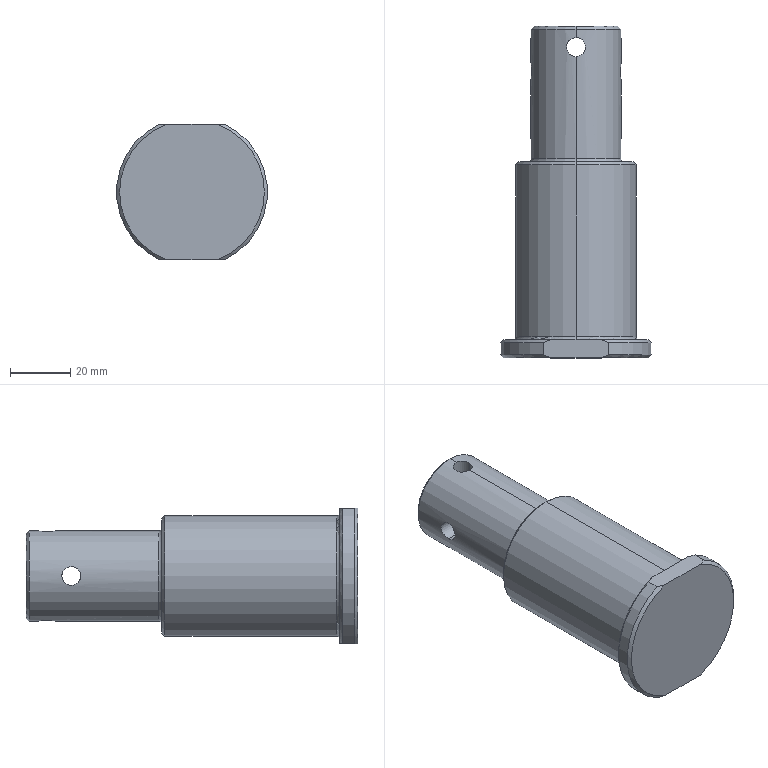Part | SolidWorks | features ICE 3, Chamfer 1, Fillet 1, Revolution 1 | 1 solid | 28 faces | box 50 x 110 x 45 mm | volume 115257 mm3 | cylinder 10 | cone 8 | plane 6 | torus 4 | commonest cylinder face diameters 6.3 x4 30 x2 40 x2 50 x2
STEP:
#1=CARTESIAN_POINT('',(-14.666,95.,3.15));
#2=VERTEX_POINT('',#1);
#3=CARTESIAN_POINT('',(-14.666,95.,-3.15));
#4=VERTEX_POINT('',#3);
#5=CARTESIAN_POINT('',(-14.666,95.,3.15));
#6=CARTESIAN_POINT('',(-14.666,94.794,3.15));
#7=CARTESIAN_POINT('',(-14.67,94.589,3.13));
#8=CARTESIAN_POINT('',(-14.687,94.181,3.049));
#9=CARTESIAN_POINT('',(-14.7,93.983,2.988));
#10=CARTESIAN_POINT('',(-14.731,93.604,2.831));
#11=CARTESIAN_POINT('',(-14.749,93.42,2.733));
#12=CARTESIAN_POINT('',(-14.79,93.077,2.504));
#13=CARTESIAN_POINT('',(-14.812,92.919,2.374));
#14=CARTESIAN_POINT('',(-14.855,92.629,2.084));
#15=CARTESIAN_POINT('',(-14.877,92.496,1.922));
#16=CARTESIAN_POINT('',(-14.917,92.268,1.581));
#17=CARTESIAN_POINT('',(-14.936,92.171,1.401));
#18=CARTESIAN_POINT('',(-14.982,91.932,0.8271));
#19=CARTESIAN_POINT('',(-15.,91.85,0.4173));
#20=CARTESIAN_POINT('',(-15.,91.85,-0.2065));
#21=CARTESIAN_POINT('',(-14.996,91.87,-0.4113));
#22=CARTESIAN_POINT('',(-14.979,91.95,-0.8152));
#23=CARTESIAN_POINT('',(-14.967,92.011,-1.016));
#24=CARTESIAN_POINT('',(-14.936,92.169,-1.397));
#25=CARTESIAN_POINT('',(-14.918,92.266,-1.577));
#26=CARTESIAN_POINT('',(-14.878,92.495,-1.92));
#27=CARTESIAN_POINT('',(-14.856,92.627,-2.081));
#28=CARTESIAN_POINT('',(-14.79,93.061,-2.516));
#29=CARTESIAN_POINT('',(-14.747,93.411,-2.75));
#30=CARTESIAN_POINT('',(-14.7,93.979,-2.987));
#31=CARTESIAN_POINT('',(-14.687,94.179,-3.048));
#32=CARTESIAN_POINT('',(-14.67,94.585,-3.129));
#33=CARTESIAN_POINT('',(-14.666,94.791,-3.15));
#34=CARTESIAN_POINT('',(-14.666,95.,-3.15));
#35=B_SPLINE_CURVE_WITH_KNOTS('',3,(#5,#6,#7,#8,#9,#10,#11,#12,#13,#14,#15,#16,#17,#18,#19,#20,#21,#22,#23,#24,#25,#26,#27,#28,#29,#30,#31,#32,#33,#34),.UNSPECIFIED.,.F.,.F.,(4,2,2,2,2,2,2,2,2,2,2,2,2,2,4),(0.009876,0.01049,0.01111,0.01173,0.01234,0.01296,0.01358,0.01481,0.01543,0.01605,0.01666,0.01728,0.01851,0.01913,0.01975),.UNSPECIFIED.);
#36=EDGE_CURVE('',#2,#4,#35,.T.);
#37=ORIENTED_EDGE('',*,*,#36,.F.);
#38=CARTESIAN_POINT('',(14.666,95.,3.15));
#39=VERTEX_POINT('',#38);
#40=CARTESIAN_POINT('',(-25.,95.,3.15));
#41=DIRECTION('',(1.,0.,0.));
#42=VECTOR('',#41,1000.);
#43=LINE('',#40,#42);
#44=EDGE_CURVE('',#2,#39,#43,.T.);
#45=ORIENTED_EDGE('',*,*,#44,.T.);
#46=CARTESIAN_POINT('',(14.666,95.,-3.15));
#47=VERTEX_POINT('',#46);
#48=CARTESIAN_POINT('',(14.666,95.,-3.15));
#49=CARTESIAN_POINT('',(14.666,94.791,-3.15));
#50=CARTESIAN_POINT('',(14.67,94.586,-3.129));
#51=CARTESIAN_POINT('',(14.687,94.183,-3.049));
#52=CARTESIAN_POINT('',(14.7,93.982,-2.988));
#53=CARTESIAN_POINT('',(14.731,93.601,-2.83));
#54=CARTESIAN_POINT('',(14.749,93.42,-2.733));
#55=CARTESIAN_POINT('',(14.79,93.078,-2.504));
#56=CARTESIAN_POINT('',(14.812,92.917,-2.372));
#57=CARTESIAN_POINT('',(14.856,92.627,-2.082));
#58=CARTESIAN_POINT('',(14.877,92.497,-1.924));
#59=CARTESIAN_POINT('',(14.918,92.267,-1.58));
#60=CARTESIAN_POINT('',(14.936,92.169,-1.397));
#61=CARTESIAN_POINT('',(14.967,92.012,-1.018));
#62=CARTESIAN_POINT('',(14.979,91.951,-0.8191));
#63=CARTESIAN_POINT('',(14.996,91.87,-0.4121));
#64=CARTESIAN_POINT('',(15.,91.85,-0.2073));
#65=CARTESIAN_POINT('',(15.,91.85,0.2049));
#66=CARTESIAN_POINT('',(14.996,91.871,0.4143));
#67=CARTESIAN_POINT('',(14.979,91.951,0.8188));
#68=CARTESIAN_POINT('',(14.967,92.011,1.015));
#69=CARTESIAN_POINT('',(14.936,92.169,1.398));
#70=CARTESIAN_POINT('',(14.917,92.268,1.581));
#71=CARTESIAN_POINT('',(14.877,92.496,1.922));
#72=CARTESIAN_POINT('',(14.856,92.627,2.081));
#73=CARTESIAN_POINT('',(14.812,92.919,2.374));
#74=CARTESIAN_POINT('',(14.79,93.078,2.504));
#75=CARTESIAN_POINT('',(14.75,93.418,2.732));
#76=CARTESIAN_POINT('',(14.731,93.603,2.831));
#77=CARTESIAN_POINT('',(14.699,93.984,2.989));
#78=CARTESIAN_POINT('',(14.687,94.18,3.048));
#79=CARTESIAN_POINT('',(14.67,94.585,3.129));
#80=CARTESIAN_POINT('',(14.666,94.794,3.15));
#81=CARTESIAN_POINT('',(14.666,95.,3.15));
#82=B_SPLINE_CURVE_WITH_KNOTS('',3,(#48,#49,#50,#51,#52,#53,#54,#55,#56,#57,#58,#59,#60,#61,#62,#63,#64,#65,#66,#67,#68,#69,#70,#71,#72,#73,#74,#75,#76,#77,#78,#79,#80,#81),.UNSPECIFIED.,.F.,.F.,(4,2,2,2,2,2,2,2,2,2,2,2,2,2,2,2,4),(0.,0.0006172,0.001234,0.001852,0.002469,0.003086,0.003703,0.004321,0.004938,0.005555,0.006172,0.00679,0.007407,0.008024,0.008641,0.009259,0.009876),.UNSPECIFIED.);
#83=EDGE_CURVE('',#47,#39,#82,.T.);
#84=ORIENTED_EDGE('',*,*,#83,.F.);
#85=CARTESIAN_POINT('',(-25.,95.,-3.15));
#86=DIRECTION('',(1.,0.,0.));
#87=VECTOR('',#86,1000.);
#88=LINE('',#85,#87);
#89=EDGE_CURVE('',#4,#47,#88,.T.);
#90=ORIENTED_EDGE('',*,*,#89,.F.);
#91=EDGE_LOOP('',(#37,#45,#84,#90));
#92=FACE_OUTER_BOUND('',#91,.T.);
#93=CARTESIAN_POINT('',(-25.,95.,0.));
#94=DIRECTION('',(1.,0.,0.));
#95=DIRECTION('',(0.,0.,-1.));
#96=AXIS2_PLACEMENT_3D('',#93,#94,#95);
#97=CYLINDRICAL_SURFACE('',#96,3.15);
#98=ADVANCED_FACE('',(#92),#97,.F.);
#99=CARTESIAN_POINT('',(-3.15,103.,-14.666));
#100=VERTEX_POINT('',#99);
#101=CARTESIAN_POINT('',(0.,99.85,-15.));
#102=VERTEX_POINT('',#101);
#103=CARTESIAN_POINT('',(-3.15,103.,-14.666));
#104=CARTESIAN_POINT('',(-3.15,102.794,-14.666));
#105=CARTESIAN_POINT('',(-3.13,102.589,-14.67));
#106=CARTESIAN_POINT('',(-3.049,102.181,-14.687));
#107=CARTESIAN_POINT('',(-2.988,101.983,-14.7));
#108=CARTESIAN_POINT('',(-2.831,101.604,-14.731));
#109=CARTESIAN_POINT('',(-2.733,101.42,-14.749));
#110=CARTESIAN_POINT('',(-2.503,101.077,-14.79));
#111=CARTESIAN_POINT('',(-2.373,100.919,-14.812));
#112=CARTESIAN_POINT('',(-2.083,100.628,-14.855));
#113=CARTESIAN_POINT('',(-1.921,100.495,-14.877));
#114=CARTESIAN_POINT('',(-1.58,100.267,-14.918));
#115=CARTESIAN_POINT('',(-1.4,100.17,-14.936));
#116=CARTESIAN_POINT('',(-0.8259,99.932,-14.982));
#117=CARTESIAN_POINT('',(-0.4159,99.85,-15.));
#118=CARTESIAN_POINT('',(0.,99.85,-15.));
#119=B_SPLINE_CURVE_WITH_KNOTS('',3,(#103,#104,#105,#106,#107,#108,#109,#110,#111,#112,#113,#114,#115,#116,#117,#118),.UNSPECIFIED.,.F.,.F.,(4,2,2,2,2,2,2,4),(0.009876,0.01049,0.01111,0.01173,0.01234,0.01296,0.01358,0.01481),.UNSPECIFIED.);
#120=EDGE_CURVE('',#100,#102,#119,.T.);
#121=ORIENTED_EDGE('',*,*,#120,.F.);
#122=CARTESIAN_POINT('',(-3.15,103.,14.666));
#123=VERTEX_POINT('',#122);
#124=CARTESIAN_POINT('',(-3.15,103.,-22.5));
#125=DIRECTION('',(0.,0.,1.));
#126=VECTOR('',#125,1000.);
#127=LINE('',#124,#126);
#128=EDGE_CURVE('',#100,#123,#127,.T.);
#129=ORIENTED_EDGE('',*,*,#128,.T.);
#130=CARTESIAN_POINT('',(0.,99.85,15.));
#131=VERTEX_POINT('',#130);
#132=CARTESIAN_POINT('',(0.,99.85,15.));
#133=CARTESIAN_POINT('',(-0.2088,99.85,15.));
#134=CARTESIAN_POINT('',(-0.414,99.871,14.996));
#135=CARTESIAN_POINT('',(-0.8175,99.951,14.979));
#136=CARTESIAN_POINT('',(-1.018,100.012,14.967));
#137=CARTESIAN_POINT('',(-1.399,100.17,14.936));
#138=CARTESIAN_POINT('',(-1.58,100.267,14.918));
#139=CARTESIAN_POINT('',(-1.922,100.496,14.877));
#140=CARTESIAN_POINT('',(-2.084,100.629,14.855));
#141=CARTESIAN_POINT('',(-2.373,100.919,14.812));
#142=CARTESIAN_POINT('',(-2.503,101.077,14.79));
#143=CARTESIAN_POINT('',(-2.734,101.421,14.749));
#144=CARTESIAN_POINT('',(-2.831,101.604,14.731));
#145=CARTESIAN_POINT('',(-2.988,101.983,14.7));
#146=CARTESIAN_POINT('',(-3.049,102.182,14.687));
#147=CARTESIAN_POINT('',(-3.13,102.589,14.67));
#148=CARTESIAN_POINT('',(-3.15,102.794,14.666));
#149=CARTESIAN_POINT('',(-3.15,103.,14.666));
#150=B_SPLINE_CURVE_WITH_KNOTS('',3,(#132,#133,#134,#135,#136,#137,#138,#139,#140,#141,#142,#143,#144,#145,#146,#147,#148,#149),.UNSPECIFIED.,.F.,.F.,(4,2,2,2,2,2,2,2,4),(0.,0.0006174,0.001235,0.001852,0.00247,0.003087,0.003704,0.004322,0.004939),.UNSPECIFIED.);
#151=EDGE_CURVE('',#131,#123,#150,.T.);
#152=ORIENTED_EDGE('',*,*,#151,.F.);
#153=CARTESIAN_POINT('',(3.15,103.,14.666));
#154=VERTEX_POINT('',#153);
#155=CARTESIAN_POINT('',(3.15,103.,14.666));
#156=CARTESIAN_POINT('',(3.15,102.792,14.666));
#157=CARTESIAN_POINT('',(3.13,102.587,14.67));
#158=CARTESIAN_POINT('',(3.049,102.184,14.687));
#159=CARTESIAN_POINT('',(2.988,101.983,14.7));
#160=CARTESIAN_POINT('',(2.831,101.603,14.731));
#161=CARTESIAN_POINT('',(2.734,101.422,14.749));
#162=CARTESIAN_POINT('',(2.505,101.079,14.79));
#163=CARTESIAN_POINT('',(2.373,100.918,14.812));
#164=CARTESIAN_POINT('',(1.939,100.484,14.877));
#165=CARTESIAN_POINT('',(1.589,100.249,14.92));
#166=CARTESIAN_POINT('',(1.021,100.013,14.966));
#167=CARTESIAN_POINT('',(0.8208,99.952,14.979));
#168=CARTESIAN_POINT('',(0.4145,99.871,14.996));
#169=CARTESIAN_POINT('',(0.2086,99.85,15.));
#170=CARTESIAN_POINT('',(0.,99.85,15.));
#171=B_SPLINE_CURVE_WITH_KNOTS('',3,(#155,#156,#157,#158,#159,#160,#161,#162,#163,#164,#165,#166,#167,#168,#169,#170),.UNSPECIFIED.,.F.,.F.,(4,2,2,2,2,2,2,4),(0.01481,0.01543,0.01605,0.01666,0.01728,0.01852,0.01913,0.01975),.UNSPECIFIED.);
#172=EDGE_CURVE('',#154,#131,#171,.T.);
#173=ORIENTED_EDGE('',*,*,#172,.F.);
#174=CARTESIAN_POINT('',(3.15,103.,-14.666));
#175=VERTEX_POINT('',#174);
#176=CARTESIAN_POINT('',(3.15,103.,-22.5));
#177=DIRECTION('',(0.,0.,1.));
#178=VECTOR('',#177,1000.);
#179=LINE('',#176,#178);
#180=EDGE_CURVE('',#175,#154,#179,.T.);
#181=ORIENTED_EDGE('',*,*,#180,.F.);
#182=CARTESIAN_POINT('',(0.,99.85,-15.));
#183=CARTESIAN_POINT('',(0.2078,99.85,-15.));
#184=CARTESIAN_POINT('',(0.4127,99.87,-14.996));
#185=CARTESIAN_POINT('',(0.8164,99.951,-14.979));
#186=CARTESIAN_POINT('',(1.017,100.012,-14.967));
#187=CARTESIAN_POINT('',(1.397,100.169,-14.936));
#188=CARTESIAN_POINT('',(1.578,100.266,-14.918));
#189=CARTESIAN_POINT('',(1.921,100.495,-14.877));
#190=CARTESIAN_POINT('',(2.082,100.627,-14.856));
#191=CARTESIAN_POINT('',(2.516,101.061,-14.79));
#192=CARTESIAN_POINT('',(2.751,101.411,-14.747));
#193=CARTESIAN_POINT('',(2.987,101.979,-14.7));
#194=CARTESIAN_POINT('',(3.048,102.179,-14.687));
#195=CARTESIAN_POINT('',(3.129,102.585,-14.67));
#196=CARTESIAN_POINT('',(3.15,102.791,-14.666));
#197=CARTESIAN_POINT('',(3.15,103.,-14.666));
#198=B_SPLINE_CURVE_WITH_KNOTS('',3,(#182,#183,#184,#185,#186,#187,#188,#189,#190,#191,#192,#193,#194,#195,#196,#197),.UNSPECIFIED.,.F.,.F.,(4,2,2,2,2,2,2,4),(0.01481,0.01543,0.01605,0.01666,0.01728,0.01852,0.01913,0.01975),.UNSPECIFIED.);
#199=EDGE_CURVE('',#102,#175,#198,.T.);
#200=ORIENTED_EDGE('',*,*,#199,.F.);
#201=EDGE_LOOP('',(#121,#129,#152,#173,#181,#200));
#202=FACE_OUTER_BOUND('',#201,.T.);
#203=CARTESIAN_POINT('',(0.,103.,-22.5));
#204=DIRECTION('',(0.,0.,1.));
#205=DIRECTION('',(1.,0.,0.));
#206=AXIS2_PLACEMENT_3D('',#203,#204,#205);
#207=CYLINDRICAL_SURFACE('',#206,3.15);
#208=ADVANCED_FACE('',(#202),#207,.F.);
#209=CARTESIAN_POINT('',(0.,6.,21.));
#210=VERTEX_POINT('',#209);
#211=CARTESIAN_POINT('',(0.,6.,-21.));
#212=VERTEX_POINT('',#211);
#213=CARTESIAN_POINT('',(0.,6.,0.));
#214=DIRECTION('',(0.,-1.,0.));
#215=DIRECTION('',(0.,0.,-1.));
#216=AXIS2_PLACEMENT_3D('',#213,#214,#215);
#217=CIRCLE('',#216,21.);
#218=EDGE_CURVE('',#210,#212,#217,.T.);
#219=ORIENTED_EDGE('',*,*,#218,.F.);
#220=CARTESIAN_POINT('',(0.,7.,20.));
#221=VERTEX_POINT('',#220);
#222=CARTESIAN_POINT('',(0.,7.,21.));
#223=DIRECTION('',(1.,0.,0.));
#224=DIRECTION('',(0.,0.,-1.));
#225=AXIS2_PLACEMENT_3D('',#222,#223,#224);
#226=CIRCLE('',#225,1.);
#227=EDGE_CURVE('',#210,#221,#226,.T.);
#228=ORIENTED_EDGE('',*,*,#227,.T.);
#229=CARTESIAN_POINT('',(0.,7.,-20.));
#230=VERTEX_POINT('',#229);
#231=CARTESIAN_POINT('',(0.,7.,0.));
#232=DIRECTION('',(0.,1.,0.));
#233=DIRECTION('',(0.,0.,-1.));
#234=AXIS2_PLACEMENT_3D('',#231,#232,#233);
#235=CIRCLE('',#234,20.);
#236=EDGE_CURVE('',#230,#221,#235,.T.);
#237=ORIENTED_EDGE('',*,*,#236,.F.);
#238=CARTESIAN_POINT('',(0.,7.,-21.));
#239=DIRECTION('',(-1.,0.,0.));
#240=DIRECTION('',(0.,0.,1.));
#241=AXIS2_PLACEMENT_3D('',#238,#239,#240);
#242=CIRCLE('',#241,1.);
#243=EDGE_CURVE('',#212,#230,#242,.T.);
#244=ORIENTED_EDGE('',*,*,#243,.F.);
#245=EDGE_LOOP('',(#219,#228,#237,#244));
#246=FACE_OUTER_BOUND('',#245,.T.);
#247=CARTESIAN_POINT('',(0.,7.,0.));
#248=DIRECTION('',(0.,-1.,0.));
#249=DIRECTION('',(0.,0.,-1.));
#250=AXIS2_PLACEMENT_3D('',#247,#248,#249);
#251=TOROIDAL_SURFACE('',#250,21.,1.);
#252=ADVANCED_FACE('',(#246),#251,.F.);
#253=CARTESIAN_POINT('',(0.,65.,16.));
#254=VERTEX_POINT('',#253);
#255=CARTESIAN_POINT('',(0.,65.,-16.));
#256=VERTEX_POINT('',#255);
#257=CARTESIAN_POINT('',(0.,65.,0.));
#258=DIRECTION('',(0.,-1.,0.));
#259=DIRECTION('',(0.,0.,-1.));
#260=AXIS2_PLACEMENT_3D('',#257,#258,#259);
#261=CIRCLE('',#260,16.);
#262=EDGE_CURVE('',#254,#256,#261,.T.);
#263=ORIENTED_EDGE('',*,*,#262,.F.);
#264=CARTESIAN_POINT('',(0.,66.,15.));
#265=VERTEX_POINT('',#264);
#266=CARTESIAN_POINT('',(0.,66.,16.));
#267=DIRECTION('',(1.,0.,0.));
#268=DIRECTION('',(0.,0.,-1.));
#269=AXIS2_PLACEMENT_3D('',#266,#267,#268);
#270=CIRCLE('',#269,1.);
#271=EDGE_CURVE('',#254,#265,#270,.T.);
#272=ORIENTED_EDGE('',*,*,#271,.T.);
#273=CARTESIAN_POINT('',(0.,66.,-15.));
#274=VERTEX_POINT('',#273);
#275=CARTESIAN_POINT('',(0.,66.,0.));
#276=DIRECTION('',(0.,1.,0.));
#277=DIRECTION('',(0.,0.,-1.));
#278=AXIS2_PLACEMENT_3D('',#275,#276,#277);
#279=CIRCLE('',#278,15.);
#280=EDGE_CURVE('',#274,#265,#279,.T.);
#281=ORIENTED_EDGE('',*,*,#280,.F.);
#282=CARTESIAN_POINT('',(0.,66.,-16.));
#283=DIRECTION('',(-1.,0.,0.));
#284=DIRECTION('',(0.,0.,1.));
#285=AXIS2_PLACEMENT_3D('',#282,#283,#284);
#286=CIRCLE('',#285,1.);
#287=EDGE_CURVE('',#256,#274,#286,.T.);
#288=ORIENTED_EDGE('',*,*,#287,.F.);
#289=EDGE_LOOP('',(#263,#272,#281,#288));
#290=FACE_OUTER_BOUND('',#289,.T.);
#291=CARTESIAN_POINT('',(0.,66.,0.));
#292=DIRECTION('',(0.,-1.,0.));
#293=DIRECTION('',(0.,0.,-1.));
#294=AXIS2_PLACEMENT_3D('',#291,#292,#293);
#295=TOROIDAL_SURFACE('',#294,16.,1.);
#296=ADVANCED_FACE('',(#290),#295,.F.);
#297=CARTESIAN_POINT('',(0.,65.,19.));
#298=VERTEX_POINT('',#297);
#299=CARTESIAN_POINT('',(0.,65.,-19.));
#300=VERTEX_POINT('',#299);
#301=CARTESIAN_POINT('',(0.,65.,0.));
#302=DIRECTION('',(0.,1.,0.));
#303=DIRECTION('',(0.,0.,-1.));
#304=AXIS2_PLACEMENT_3D('',#301,#302,#303);
#305=CIRCLE('',#304,19.);
#306=EDGE_CURVE('',#298,#300,#305,.T.);
#307=ORIENTED_EDGE('',*,*,#306,.F.);
#308=CARTESIAN_POINT('',(0.,64.,20.));
#309=VERTEX_POINT('',#308);
#310=CARTESIAN_POINT('',(0.,65.,19.));
#311=DIRECTION('',(0.,-0.7071,0.7071));
#312=VECTOR('',#311,1000.);
#313=LINE('',#310,#312);
#314=EDGE_CURVE('',#298,#309,#313,.T.);
#315=ORIENTED_EDGE('',*,*,#314,.T.);
#316=CARTESIAN_POINT('',(0.,64.,-20.));
#317=VERTEX_POINT('',#316);
#318=CARTESIAN_POINT('',(0.,64.,0.));
#319=DIRECTION('',(0.,-1.,0.));
#320=DIRECTION('',(0.,0.,-1.));
#321=AXIS2_PLACEMENT_3D('',#318,#319,#320);
#322=CIRCLE('',#321,20.);
#323=EDGE_CURVE('',#317,#309,#322,.T.);
#324=ORIENTED_EDGE('',*,*,#323,.F.);
#325=CARTESIAN_POINT('',(0.,65.,-19.));
#326=DIRECTION('',(0.,-0.7071,-0.7071));
#327=VECTOR('',#326,1000.);
#328=LINE('',#325,#327);
#329=EDGE_CURVE('',#300,#317,#328,.T.);
#330=ORIENTED_EDGE('',*,*,#329,.F.);
#331=EDGE_LOOP('',(#307,#315,#324,#330));
#332=FACE_OUTER_BOUND('',#331,.T.);
#333=CARTESIAN_POINT('',(0.,65.,0.));
#334=DIRECTION('',(0.,-1.,0.));
#335=DIRECTION('',(0.,0.,-1.));
#336=AXIS2_PLACEMENT_3D('',#333,#334,#335);
#337=CONICAL_SURFACE('',#336,19.,0.7854);
#338=ADVANCED_FACE('',(#332),#337,.T.);
#339=CARTESIAN_POINT('',(0.,110.,14.));
#340=VERTEX_POINT('',#339);
#341=CARTESIAN_POINT('',(0.,110.,-14.));
#342=VERTEX_POINT('',#341);
#343=CARTESIAN_POINT('',(0.,110.,0.));
#344=DIRECTION('',(0.,1.,0.));
#345=DIRECTION('',(0.,0.,-1.));
#346=AXIS2_PLACEMENT_3D('',#343,#344,#345);
#347=CIRCLE('',#346,14.);
#348=EDGE_CURVE('',#340,#342,#347,.T.);
#349=ORIENTED_EDGE('',*,*,#348,.F.);
#350=CARTESIAN_POINT('',(0.,109.,15.));
#351=VERTEX_POINT('',#350);
#352=CARTESIAN_POINT('',(0.,110.,14.));
#353=DIRECTION('',(0.,-0.7071,0.7071));
#354=VECTOR('',#353,1000.);
#355=LINE('',#352,#354);
#356=EDGE_CURVE('',#340,#351,#355,.T.);
#357=ORIENTED_EDGE('',*,*,#356,.T.);
#358=CARTESIAN_POINT('',(0.,109.,-15.));
#359=VERTEX_POINT('',#358);
#360=CARTESIAN_POINT('',(0.,109.,0.));
#361=DIRECTION('',(0.,-1.,0.));
#362=DIRECTION('',(0.,0.,-1.));
#363=AXIS2_PLACEMENT_3D('',#360,#361,#362);
#364=CIRCLE('',#363,15.);
#365=EDGE_CURVE('',#359,#351,#364,.T.);
#366=ORIENTED_EDGE('',*,*,#365,.F.);
#367=CARTESIAN_POINT('',(0.,110.,-14.));
#368=DIRECTION('',(0.,-0.7071,-0.7071));
#369=VECTOR('',#368,1000.);
#370=LINE('',#367,#369);
#371=EDGE_CURVE('',#342,#359,#370,.T.);
#372=ORIENTED_EDGE('',*,*,#371,.F.);
#373=EDGE_LOOP('',(#349,#357,#366,#372));
#374=FACE_OUTER_BOUND('',#373,.T.);
#375=CARTESIAN_POINT('',(0.,110.,0.));
#376=DIRECTION('',(0.,-1.,0.));
#377=DIRECTION('',(0.,0.,-1.));
#378=AXIS2_PLACEMENT_3D('',#375,#376,#377);
#379=CONICAL_SURFACE('',#378,14.,0.7854);
#380=ADVANCED_FACE('',(#374),#379,.T.);
#381=ORIENTED_EDGE('',*,*,#83,.T.);
#382=CARTESIAN_POINT('',(14.666,95.,3.15));
#383=CARTESIAN_POINT('',(14.666,95.206,3.15));
#384=CARTESIAN_POINT('',(14.67,95.411,3.13));
#385=CARTESIAN_POINT('',(14.687,95.819,3.049));
#386=CARTESIAN_POINT('',(14.7,96.017,2.988));
#387=CARTESIAN_POINT('',(14.731,96.396,2.831));
#388=CARTESIAN_POINT('',(14.749,96.58,2.733));
#389=CARTESIAN_POINT('',(14.79,96.923,2.504));
#390=CARTESIAN_POINT('',(14.812,97.081,2.374));
#391=CARTESIAN_POINT('',(14.855,97.371,2.084));
#392=CARTESIAN_POINT('',(14.877,97.504,1.922));
#393=CARTESIAN_POINT('',(14.917,97.732,1.581));
#394=CARTESIAN_POINT('',(14.936,97.829,1.401));
#395=CARTESIAN_POINT('',(14.982,98.068,0.8271));
#396=CARTESIAN_POINT('',(15.,98.15,0.4173));
#397=CARTESIAN_POINT('',(15.,98.15,-0.2065));
#398=CARTESIAN_POINT('',(14.996,98.13,-0.4113));
#399=CARTESIAN_POINT('',(14.979,98.05,-0.8152));
#400=CARTESIAN_POINT('',(14.967,97.989,-1.016));
#401=CARTESIAN_POINT('',(14.936,97.831,-1.397));
#402=CARTESIAN_POINT('',(14.918,97.734,-1.577));
#403=CARTESIAN_POINT('',(14.878,97.505,-1.92));
#404=CARTESIAN_POINT('',(14.856,97.373,-2.081));
#405=CARTESIAN_POINT('',(14.79,96.939,-2.516));
#406=CARTESIAN_POINT('',(14.747,96.589,-2.75));
#407=CARTESIAN_POINT('',(14.7,96.021,-2.987));
#408=CARTESIAN_POINT('',(14.687,95.821,-3.048));
#409=CARTESIAN_POINT('',(14.67,95.415,-3.129));
#410=CARTESIAN_POINT('',(14.666,95.209,-3.15));
#411=CARTESIAN_POINT('',(14.666,95.,-3.15));
#412=B_SPLINE_CURVE_WITH_KNOTS('',3,(#382,#383,#384,#385,#386,#387,#388,#389,#390,#391,#392,#393,#394,#395,#396,#397,#398,#399,#400,#401,#402,#403,#404,#405,#406,#407,#408,#409,#410,#411),.UNSPECIFIED.,.F.,.F.,(4,2,2,2,2,2,2,2,2,2,2,2,2,2,4),(0.009876,0.01049,0.01111,0.01173,0.01234,0.01296,0.01358,0.01481,0.01543,0.01605,0.01666,0.01728,0.01851,0.01913,0.01975),.UNSPECIFIED.);
#413=EDGE_CURVE('',#39,#47,#412,.T.);
#414=ORIENTED_EDGE('',*,*,#413,.T.);
#415=EDGE_LOOP('',(#381,#414));
#416=FACE_BOUND('',#415,.T.);
#417=CARTESIAN_POINT('',(0.,66.,0.));
#418=DIRECTION('',(0.,1.,0.));
#419=DIRECTION('',(0.,0.,-1.));
#420=AXIS2_PLACEMENT_3D('',#417,#418,#419);
#421=CIRCLE('',#420,15.);
#422=EDGE_CURVE('',#265,#274,#421,.T.);
#423=ORIENTED_EDGE('',*,*,#422,.T.);
#424=CARTESIAN_POINT('',(0.,0.,-15.));
#425=DIRECTION('',(0.,1.,0.));
#426=VECTOR('',#425,1000.);
#427=LINE('',#424,#426);
#428=EDGE_CURVE('',#274,#102,#427,.T.);
#429=ORIENTED_EDGE('',*,*,#428,.T.);
#430=ORIENTED_EDGE('',*,*,#199,.T.);
#431=CARTESIAN_POINT('',(0.,106.15,-15.));
#432=VERTEX_POINT('',#431);
#433=CARTESIAN_POINT('',(3.15,103.,-14.666));
#434=CARTESIAN_POINT('',(3.15,103.209,-14.666));
#435=CARTESIAN_POINT('',(3.129,103.414,-14.67));
#436=CARTESIAN_POINT('',(3.049,103.818,-14.687));
#437=CARTESIAN_POINT('',(2.988,104.018,-14.7));
#438=CARTESIAN_POINT('',(2.83,104.399,-14.731));
#439=CARTESIAN_POINT('',(2.733,104.58,-14.749));
#440=CARTESIAN_POINT('',(2.504,104.922,-14.79));
#441=CARTESIAN_POINT('',(2.371,105.083,-14.812));
#442=CARTESIAN_POINT('',(2.082,105.373,-14.856));
#443=CARTESIAN_POINT('',(1.923,105.503,-14.877));
#444=CARTESIAN_POINT('',(1.579,105.734,-14.918));
#445=CARTESIAN_POINT('',(1.396,105.831,-14.936));
#446=CARTESIAN_POINT('',(1.017,105.988,-14.967));
#447=CARTESIAN_POINT('',(0.8181,106.049,-14.979));
#448=CARTESIAN_POINT('',(0.411,106.13,-14.996));
#449=CARTESIAN_POINT('',(0.2062,106.15,-15.));
#450=CARTESIAN_POINT('',(0.,106.15,-15.));
#451=B_SPLINE_CURVE_WITH_KNOTS('',3,(#433,#434,#435,#436,#437,#438,#439,#440,#441,#442,#443,#444,#445,#446,#447,#448,#449,#450),.UNSPECIFIED.,.F.,.F.,(4,2,2,2,2,2,2,2,4),(0.,0.0006174,0.001235,0.001852,0.00247,0.003087,0.003704,0.004322,0.004939),.UNSPECIFIED.);
#452=EDGE_CURVE('',#175,#432,#451,.T.);
#453=ORIENTED_EDGE('',*,*,#452,.T.);
#454=CARTESIAN_POINT('',(0.,0.,-15.));
#455=DIRECTION('',(0.,1.,0.));
#456=VECTOR('',#455,1000.);
#457=LINE('',#454,#456);
#458=EDGE_CURVE('',#432,#359,#457,.T.);
#459=ORIENTED_EDGE('',*,*,#458,.T.);
#460=ORIENTED_EDGE('',*,*,#365,.T.);
#461=CARTESIAN_POINT('',(0.,106.15,15.));
#462=VERTEX_POINT('',#461);
#463=CARTESIAN_POINT('',(0.,0.,15.));
#464=DIRECTION('',(0.,1.,0.));
#465=VECTOR('',#464,1000.);
#466=LINE('',#463,#465);
#467=EDGE_CURVE('',#462,#351,#466,.T.);
#468=ORIENTED_EDGE('',*,*,#467,.F.);
#469=CARTESIAN_POINT('',(0.,106.15,15.));
#470=CARTESIAN_POINT('',(0.2059,106.15,15.));
#471=CARTESIAN_POINT('',(0.411,106.13,14.996));
#472=CARTESIAN_POINT('',(0.8194,106.049,14.979));
#473=CARTESIAN_POINT('',(1.017,105.988,14.967));
#474=CARTESIAN_POINT('',(1.396,105.831,14.936));
#475=CARTESIAN_POINT('',(1.581,105.733,14.917));
#476=CARTESIAN_POINT('',(1.923,105.503,14.877));
#477=CARTESIAN_POINT('',(2.081,105.373,14.856));
#478=CARTESIAN_POINT('',(2.372,105.083,14.812));
#479=CARTESIAN_POINT('',(2.505,104.921,14.79));
#480=CARTESIAN_POINT('',(2.733,104.58,14.749));
#481=CARTESIAN_POINT('',(2.83,104.4,14.731));
#482=CARTESIAN_POINT('',(3.068,103.826,14.684));
#483=CARTESIAN_POINT('',(3.15,103.416,14.666));
#484=CARTESIAN_POINT('',(3.15,103.,14.666));
#485=B_SPLINE_CURVE_WITH_KNOTS('',3,(#469,#470,#471,#472,#473,#474,#475,#476,#477,#478,#479,#480,#481,#482,#483,#484),.UNSPECIFIED.,.F.,.F.,(4,2,2,2,2,2,2,4),(0.009876,0.01049,0.01111,0.01173,0.01234,0.01296,0.01358,0.01481),.UNSPECIFIED.);
#486=EDGE_CURVE('',#462,#154,#485,.T.);
#487=ORIENTED_EDGE('',*,*,#486,.T.);
#488=ORIENTED_EDGE('',*,*,#172,.T.);
#489=CARTESIAN_POINT('',(0.,0.,15.));
#490=DIRECTION('',(0.,1.,0.));
#491=VECTOR('',#490,1000.);
#492=LINE('',#489,#491);
#493=EDGE_CURVE('',#265,#131,#492,.T.);
#494=ORIENTED_EDGE('',*,*,#493,.F.);
#495=EDGE_LOOP('',(#423,#429,#430,#453,#459,#460,#468,#487,#488,#494));
#496=FACE_OUTER_BOUND('',#495,.T.);
#497=CARTESIAN_POINT('',(0.,0.,0.));
#498=DIRECTION('',(0.,1.,0.));
#499=DIRECTION('',(0.,0.,1.));
#500=AXIS2_PLACEMENT_3D('',#497,#498,#499);
#501=CYLINDRICAL_SURFACE('',#500,15.);
#502=ADVANCED_FACE('',(#416,#496),#501,.T.);
#503=CARTESIAN_POINT('',(0.,7.,0.));
#504=DIRECTION('',(0.,1.,0.));
#505=DIRECTION('',(0.,0.,-1.));
#506=AXIS2_PLACEMENT_3D('',#503,#504,#505);
#507=CIRCLE('',#506,20.);
#508=EDGE_CURVE('',#221,#230,#507,.T.);
#509=ORIENTED_EDGE('',*,*,#508,.T.);
#510=CARTESIAN_POINT('',(0.,0.,-20.));
#511=DIRECTION('',(0.,1.,0.));
#512=VECTOR('',#511,1000.);
#513=LINE('',#510,#512);
#514=EDGE_CURVE('',#230,#317,#513,.T.);
#515=ORIENTED_EDGE('',*,*,#514,.T.);
#516=ORIENTED_EDGE('',*,*,#323,.T.);
#517=CARTESIAN_POINT('',(0.,0.,20.));
#518=DIRECTION('',(0.,1.,0.));
#519=VECTOR('',#518,1000.);
#520=LINE('',#517,#519);
#521=EDGE_CURVE('',#221,#309,#520,.T.);
#522=ORIENTED_EDGE('',*,*,#521,.F.);
#523=EDGE_LOOP('',(#509,#515,#516,#522));
#524=FACE_OUTER_BOUND('',#523,.T.);
#525=CARTESIAN_POINT('',(0.,0.,0.));
#526=DIRECTION('',(0.,1.,0.));
#527=DIRECTION('',(0.,0.,1.));
#528=AXIS2_PLACEMENT_3D('',#525,#526,#527);
#529=CYLINDRICAL_SURFACE('',#528,20.);
#530=ADVANCED_FACE('',(#524),#529,.T.);
#531=CARTESIAN_POINT('',(-10.897,1.,-22.5));
#532=VERTEX_POINT('',#531);
#533=CARTESIAN_POINT('',(-10.897,1.,22.5));
#534=VERTEX_POINT('',#533);
#535=CARTESIAN_POINT('',(0.,1.,0.));
#536=DIRECTION('',(0.,1.,0.));
#537=DIRECTION('',(0.,0.,1.));
#538=AXIS2_PLACEMENT_3D('',#535,#536,#537);
#539=CIRCLE('',#538,25.);
#540=EDGE_CURVE('',#532,#534,#539,.T.);
#541=ORIENTED_EDGE('',*,*,#540,.T.);
#542=CARTESIAN_POINT('',(-10.897,5.,22.5));
#543=VERTEX_POINT('',#542);
#544=CARTESIAN_POINT('',(-10.897,0.,22.5));
#545=DIRECTION('',(0.,1.,0.));
#546=VECTOR('',#545,1000.);
#547=LINE('',#544,#546);
#548=EDGE_CURVE('',#534,#543,#547,.T.);
#549=ORIENTED_EDGE('',*,*,#548,.T.);
#550=CARTESIAN_POINT('',(-10.897,5.,-22.5));
#551=VERTEX_POINT('',#550);
#552=CARTESIAN_POINT('',(0.,5.,0.));
#553=DIRECTION('',(0.,-1.,0.));
#554=DIRECTION('',(0.,0.,-1.));
#555=AXIS2_PLACEMENT_3D('',#552,#553,#554);
#556=CIRCLE('',#555,25.);
#557=EDGE_CURVE('',#543,#551,#556,.T.);
#558=ORIENTED_EDGE('',*,*,#557,.T.);
#559=CARTESIAN_POINT('',(-10.897,0.,-22.5));
#560=DIRECTION('',(0.,-1.,0.));
#561=VECTOR('',#560,1000.);
#562=LINE('',#559,#561);
#563=EDGE_CURVE('',#551,#532,#562,.T.);
#564=ORIENTED_EDGE('',*,*,#563,.T.);
#565=EDGE_LOOP('',(#541,#549,#558,#564));
#566=FACE_OUTER_BOUND('',#565,.T.);
#567=CARTESIAN_POINT('',(0.,0.,0.));
#568=DIRECTION('',(0.,1.,0.));
#569=DIRECTION('',(0.,0.,1.));
#570=AXIS2_PLACEMENT_3D('',#567,#568,#569);
#571=CYLINDRICAL_SURFACE('',#570,25.);
#572=ADVANCED_FACE('',(#566),#571,.T.);
#573=CARTESIAN_POINT('',(-8.352,0.,22.5));
#574=VERTEX_POINT('',#573);
#575=CARTESIAN_POINT('',(-10.897,1.,22.5));
#576=CARTESIAN_POINT('',(-10.062,0.6359,22.5));
#577=CARTESIAN_POINT('',(-9.214,0.3002,22.5));
#578=CARTESIAN_POINT('',(-8.352,0.,22.5));
#579=B_SPLINE_CURVE_WITH_KNOTS('',3,(#575,#576,#577,#578),.UNSPECIFIED.,.F.,.F.,(4,4),(0.04963,0.05237),.UNSPECIFIED.);
#580=EDGE_CURVE('',#534,#574,#579,.T.);
#581=ORIENTED_EDGE('',*,*,#580,.F.);
#582=ORIENTED_EDGE('',*,*,#540,.F.);
#583=CARTESIAN_POINT('',(-8.352,0.,-22.5));
#584=VERTEX_POINT('',#583);
#585=CARTESIAN_POINT('',(-8.352,0.,-22.5));
#586=CARTESIAN_POINT('',(-9.212,0.2995,-22.5));
#587=CARTESIAN_POINT('',(-10.065,0.6371,-22.5));
#588=CARTESIAN_POINT('',(-10.897,1.,-22.5));
#589=B_SPLINE_CURVE_WITH_KNOTS('',3,(#585,#586,#587,#588),.UNSPECIFIED.,.F.,.F.,(4,4),(0.06941,0.07214),.UNSPECIFIED.);
#590=EDGE_CURVE('',#584,#532,#589,.T.);
#591=ORIENTED_EDGE('',*,*,#590,.F.);
#592=CARTESIAN_POINT('',(0.,0.,0.));
#593=DIRECTION('',(0.,-1.,0.));
#594=DIRECTION('',(0.,0.,1.));
#595=AXIS2_PLACEMENT_3D('',#592,#593,#594);
#596=CIRCLE('',#595,24.);
#597=EDGE_CURVE('',#574,#584,#596,.T.);
#598=ORIENTED_EDGE('',*,*,#597,.F.);
#599=EDGE_LOOP('',(#581,#582,#591,#598));
#600=FACE_OUTER_BOUND('',#599,.T.);
#601=CARTESIAN_POINT('',(0.,1.,0.));
#602=DIRECTION('',(0.,1.,0.));
#603=DIRECTION('',(0.,0.,1.));
#604=AXIS2_PLACEMENT_3D('',#601,#602,#603);
#605=CONICAL_SURFACE('',#604,25.,0.7854);
#606=ADVANCED_FACE('',(#600),#605,.T.);
#607=CARTESIAN_POINT('',(10.897,5.,22.5));
#608=VERTEX_POINT('',#607);
#609=CARTESIAN_POINT('',(8.352,6.,22.5));
#610=VERTEX_POINT('',#609);
#611=CARTESIAN_POINT('',(10.897,5.,22.5));
#612=CARTESIAN_POINT('',(10.062,5.364,22.5));
#613=CARTESIAN_POINT('',(9.214,5.7,22.5));
#614=CARTESIAN_POINT('',(8.352,6.,22.5));
#615=B_SPLINE_CURVE_WITH_KNOTS('',3,(#611,#612,#613,#614),.UNSPECIFIED.,.F.,.F.,(4,4),(0.04963,0.05237),.UNSPECIFIED.);
#616=EDGE_CURVE('',#608,#610,#615,.T.);
#617=ORIENTED_EDGE('',*,*,#616,.F.);
#618=CARTESIAN_POINT('',(10.897,5.,-22.5));
#619=VERTEX_POINT('',#618);
#620=CARTESIAN_POINT('',(0.,5.,0.));
#621=DIRECTION('',(0.,-1.,0.));
#622=DIRECTION('',(0.,0.,-1.));
#623=AXIS2_PLACEMENT_3D('',#620,#621,#622);
#624=CIRCLE('',#623,25.);
#625=EDGE_CURVE('',#619,#608,#624,.T.);
#626=ORIENTED_EDGE('',*,*,#625,.F.);
#627=CARTESIAN_POINT('',(8.352,6.,-22.5));
#628=VERTEX_POINT('',#627);
#629=CARTESIAN_POINT('',(8.352,6.,-22.5));
#630=CARTESIAN_POINT('',(9.212,5.701,-22.5));
#631=CARTESIAN_POINT('',(10.065,5.363,-22.5));
#632=CARTESIAN_POINT('',(10.897,5.,-22.5));
#633=B_SPLINE_CURVE_WITH_KNOTS('',3,(#629,#630,#631,#632),.UNSPECIFIED.,.F.,.F.,(4,4),(0.06941,0.07214),.UNSPECIFIED.);
#634=EDGE_CURVE('',#628,#619,#633,.T.);
#635=ORIENTED_EDGE('',*,*,#634,.F.);
#636=CARTESIAN_POINT('',(0.,6.,0.));
#637=DIRECTION('',(0.,1.,0.));
#638=DIRECTION('',(0.,0.,-1.));
#639=AXIS2_PLACEMENT_3D('',#636,#637,#638);
#640=CIRCLE('',#639,24.);
#641=EDGE_CURVE('',#610,#628,#640,.T.);
#642=ORIENTED_EDGE('',*,*,#641,.F.);
#643=EDGE_LOOP('',(#617,#626,#635,#642));
#644=FACE_OUTER_BOUND('',#643,.T.);
#645=CARTESIAN_POINT('',(0.,6.,0.));
#646=DIRECTION('',(0.,-1.,0.));
#647=DIRECTION('',(0.,0.,-1.));
#648=AXIS2_PLACEMENT_3D('',#645,#646,#647);
#649=CONICAL_SURFACE('',#648,24.,0.7854);
#650=ADVANCED_FACE('',(#644),#649,.T.);
#651=CARTESIAN_POINT('',(8.352,0.,-22.5));
#652=VERTEX_POINT('',#651);
#653=CARTESIAN_POINT('',(8.352,0.,22.5));
#654=VERTEX_POINT('',#653);
#655=CARTESIAN_POINT('',(0.,0.,0.));
#656=DIRECTION('',(0.,-1.,0.));
#657=DIRECTION('',(0.,0.,1.));
#658=AXIS2_PLACEMENT_3D('',#655,#656,#657);
#659=CIRCLE('',#658,24.);
#660=EDGE_CURVE('',#652,#654,#659,.T.);
#661=ORIENTED_EDGE('',*,*,#660,.T.);
#662=CARTESIAN_POINT('',(40.,0.,22.5));
#663=DIRECTION('',(1.,0.,0.));
#664=VECTOR('',#663,1000.);
#665=LINE('',#662,#664);
#666=EDGE_CURVE('',#574,#654,#665,.T.);
#667=ORIENTED_EDGE('',*,*,#666,.F.);
#668=ORIENTED_EDGE('',*,*,#597,.T.);
#669=CARTESIAN_POINT('',(40.,0.,-22.5));
#670=DIRECTION('',(-1.,0.,0.));
#671=VECTOR('',#670,1000.);
#672=LINE('',#669,#671);
#673=EDGE_CURVE('',#652,#584,#672,.T.);
#674=ORIENTED_EDGE('',*,*,#673,.F.);
#675=EDGE_LOOP('',(#661,#667,#668,#674));
#676=FACE_OUTER_BOUND('',#675,.T.);
#677=CARTESIAN_POINT('',(0.,0.,0.));
#678=DIRECTION('',(0.,1.,0.));
#679=DIRECTION('',(0.,0.,1.));
#680=AXIS2_PLACEMENT_3D('',#677,#678,#679);
#681=PLANE('',#680);
#682=ADVANCED_FACE('',(#676),#681,.F.);
#683=ORIENTED_EDGE('',*,*,#625,.T.);
#684=CARTESIAN_POINT('',(10.897,1.,22.5));
#685=VERTEX_POINT('',#684);
#686=CARTESIAN_POINT('',(10.897,0.,22.5));
#687=DIRECTION('',(0.,-1.,0.));
#688=VECTOR('',#687,1000.);
#689=LINE('',#686,#688);
#690=EDGE_CURVE('',#608,#685,#689,.T.);
#691=ORIENTED_EDGE('',*,*,#690,.T.);
#692=CARTESIAN_POINT('',(10.897,1.,-22.5));
#693=VERTEX_POINT('',#692);
#694=CARTESIAN_POINT('',(0.,1.,0.));
#695=DIRECTION('',(0.,1.,0.));
#696=DIRECTION('',(0.,0.,1.));
#697=AXIS2_PLACEMENT_3D('',#694,#695,#696);
#698=CIRCLE('',#697,25.);
#699=EDGE_CURVE('',#685,#693,#698,.T.);
#700=ORIENTED_EDGE('',*,*,#699,.T.);
#701=CARTESIAN_POINT('',(10.897,0.,-22.5));
#702=DIRECTION('',(0.,1.,0.));
#703=VECTOR('',#702,1000.);
#704=LINE('',#701,#703);
#705=EDGE_CURVE('',#693,#619,#704,.T.);
#706=ORIENTED_EDGE('',*,*,#705,.T.);
#707=EDGE_LOOP('',(#683,#691,#700,#706));
#708=FACE_OUTER_BOUND('',#707,.T.);
#709=CARTESIAN_POINT('',(0.,0.,0.));
#710=DIRECTION('',(0.,1.,0.));
#711=DIRECTION('',(0.,0.,1.));
#712=AXIS2_PLACEMENT_3D('',#709,#710,#711);
#713=CYLINDRICAL_SURFACE('',#712,25.);
#714=ADVANCED_FACE('',(#708),#713,.T.);
#715=CARTESIAN_POINT('',(0.,6.,0.));
#716=DIRECTION('',(0.,-1.,0.));
#717=DIRECTION('',(0.,0.,-1.));
#718=AXIS2_PLACEMENT_3D('',#715,#716,#717);
#719=CIRCLE('',#718,21.);
#720=EDGE_CURVE('',#212,#210,#719,.T.);
#721=ORIENTED_EDGE('',*,*,#720,.T.);
#722=ORIENTED_EDGE('',*,*,#218,.T.);
#723=EDGE_LOOP('',(#721,#722));
#724=FACE_BOUND('',#723,.T.);
#725=CARTESIAN_POINT('',(-8.352,6.,-22.5));
#726=VERTEX_POINT('',#725);
#727=CARTESIAN_POINT('',(-8.352,6.,22.5));
#728=VERTEX_POINT('',#727);
#729=CARTESIAN_POINT('',(0.,6.,0.));
#730=DIRECTION('',(0.,1.,0.));
#731=DIRECTION('',(0.,0.,-1.));
#732=AXIS2_PLACEMENT_3D('',#729,#730,#731);
#733=CIRCLE('',#732,24.);
#734=EDGE_CURVE('',#726,#728,#733,.T.);
#735=ORIENTED_EDGE('',*,*,#734,.T.);
#736=CARTESIAN_POINT('',(40.,6.,22.5));
#737=DIRECTION('',(-1.,0.,0.));
#738=VECTOR('',#737,1000.);
#739=LINE('',#736,#738);
#740=EDGE_CURVE('',#610,#728,#739,.T.);
#741=ORIENTED_EDGE('',*,*,#740,.F.);
#742=ORIENTED_EDGE('',*,*,#641,.T.);
#743=CARTESIAN_POINT('',(40.,6.,-22.5));
#744=DIRECTION('',(1.,0.,0.));
#745=VECTOR('',#744,1000.);
#746=LINE('',#743,#745);
#747=EDGE_CURVE('',#726,#628,#746,.T.);
#748=ORIENTED_EDGE('',*,*,#747,.F.);
#749=EDGE_LOOP('',(#735,#741,#742,#748));
#750=FACE_OUTER_BOUND('',#749,.T.);
#751=CARTESIAN_POINT('',(25.,6.,0.));
#752=DIRECTION('',(0.,-1.,0.));
#753=DIRECTION('',(0.,0.,-1.));
#754=AXIS2_PLACEMENT_3D('',#751,#752,#753);
#755=PLANE('',#754);
#756=ADVANCED_FACE('',(#724,#750),#755,.F.);
#757=ORIENTED_EDGE('',*,*,#514,.F.);
#758=ORIENTED_EDGE('',*,*,#236,.T.);
#759=ORIENTED_EDGE('',*,*,#521,.T.);
#760=CARTESIAN_POINT('',(0.,64.,0.));
#761=DIRECTION('',(0.,-1.,0.));
#762=DIRECTION('',(0.,0.,-1.));
#763=AXIS2_PLACEMENT_3D('',#760,#761,#762);
#764=CIRCLE('',#763,20.);
#765=EDGE_CURVE('',#309,#317,#764,.T.);
#766=ORIENTED_EDGE('',*,*,#765,.T.);
#767=EDGE_LOOP('',(#757,#758,#759,#766));
#768=FACE_OUTER_BOUND('',#767,.T.);
#769=CARTESIAN_POINT('',(0.,0.,0.));
#770=DIRECTION('',(0.,1.,0.));
#771=DIRECTION('',(0.,0.,1.));
#772=AXIS2_PLACEMENT_3D('',#769,#770,#771);
#773=CYLINDRICAL_SURFACE('',#772,20.);
#774=ADVANCED_FACE('',(#768),#773,.T.);
#775=CARTESIAN_POINT('',(0.,65.,0.));
#776=DIRECTION('',(0.,-1.,0.));
#777=DIRECTION('',(0.,0.,-1.));
#778=AXIS2_PLACEMENT_3D('',#775,#776,#777);
#779=CIRCLE('',#778,16.);
#780=EDGE_CURVE('',#256,#254,#779,.T.);
#781=ORIENTED_EDGE('',*,*,#780,.T.);
#782=ORIENTED_EDGE('',*,*,#262,.T.);
#783=EDGE_LOOP('',(#781,#782));
#784=FACE_BOUND('',#783,.T.);
#785=CARTESIAN_POINT('',(0.,65.,0.));
#786=DIRECTION('',(0.,1.,0.));
#787=DIRECTION('',(0.,0.,-1.));
#788=AXIS2_PLACEMENT_3D('',#785,#786,#787);
#789=CIRCLE('',#788,19.);
#790=EDGE_CURVE('',#300,#298,#789,.T.);
#791=ORIENTED_EDGE('',*,*,#790,.T.);
#792=ORIENTED_EDGE('',*,*,#306,.T.);
#793=EDGE_LOOP('',(#791,#792));
#794=FACE_OUTER_BOUND('',#793,.T.);
#795=CARTESIAN_POINT('',(20.,65.,0.));
#796=DIRECTION('',(0.,-1.,0.));
#797=DIRECTION('',(0.,0.,-1.));
#798=AXIS2_PLACEMENT_3D('',#795,#796,#797);
#799=PLANE('',#798);
#800=ADVANCED_FACE('',(#784,#794),#799,.F.);
#801=ORIENTED_EDGE('',*,*,#428,.F.);
#802=ORIENTED_EDGE('',*,*,#280,.T.);
#803=ORIENTED_EDGE('',*,*,#493,.T.);
#804=ORIENTED_EDGE('',*,*,#151,.T.);
#805=CARTESIAN_POINT('',(-3.15,103.,14.666));
#806=CARTESIAN_POINT('',(-3.15,103.206,14.666));
#807=CARTESIAN_POINT('',(-3.129,103.415,14.67));
#808=CARTESIAN_POINT('',(-3.048,103.82,14.687));
#809=CARTESIAN_POINT('',(-2.989,104.016,14.699));
#810=CARTESIAN_POINT('',(-2.83,104.398,14.731));
#811=CARTESIAN_POINT('',(-2.732,104.582,14.75));
#812=CARTESIAN_POINT('',(-2.504,104.922,14.79));
#813=CARTESIAN_POINT('',(-2.373,105.082,14.812));
#814=CARTESIAN_POINT('',(-2.08,105.374,14.856));
#815=CARTESIAN_POINT('',(-1.922,105.504,14.877));
#816=CARTESIAN_POINT('',(-1.581,105.732,14.917));
#817=CARTESIAN_POINT('',(-1.397,105.831,14.936));
#818=CARTESIAN_POINT('',(-1.016,105.989,14.967));
#819=CARTESIAN_POINT('',(-0.8199,106.048,14.979));
#820=CARTESIAN_POINT('',(-0.4149,106.129,14.996));
#821=CARTESIAN_POINT('',(-0.2059,106.15,15.));
#822=CARTESIAN_POINT('',(0.,106.15,15.));
#823=B_SPLINE_CURVE_WITH_KNOTS('',3,(#805,#806,#807,#808,#809,#810,#811,#812,#813,#814,#815,#816,#817,#818,#819,#820,#821,#822),.UNSPECIFIED.,.F.,.F.,(4,2,2,2,2,2,2,2,4),(0.004939,0.005556,0.006173,0.00679,0.007408,0.008025,0.008642,0.009259,0.009876),.UNSPECIFIED.);
#824=EDGE_CURVE('',#123,#462,#823,.T.);
#825=ORIENTED_EDGE('',*,*,#824,.T.);
#826=ORIENTED_EDGE('',*,*,#467,.T.);
#827=CARTESIAN_POINT('',(0.,109.,0.));
#828=DIRECTION('',(0.,-1.,0.));
#829=DIRECTION('',(0.,0.,-1.));
#830=AXIS2_PLACEMENT_3D('',#827,#828,#829);
#831=CIRCLE('',#830,15.);
#832=EDGE_CURVE('',#351,#359,#831,.T.);
#833=ORIENTED_EDGE('',*,*,#832,.T.);
#834=ORIENTED_EDGE('',*,*,#458,.F.);
#835=CARTESIAN_POINT('',(0.,106.15,-15.));
#836=CARTESIAN_POINT('',(-0.2061,106.15,-15.));
#837=CARTESIAN_POINT('',(-0.4154,106.129,-14.996));
#838=CARTESIAN_POINT('',(-0.8197,106.048,-14.979));
#839=CARTESIAN_POINT('',(-1.016,105.989,-14.967));
#840=CARTESIAN_POINT('',(-1.398,105.83,-14.936));
#841=CARTESIAN_POINT('',(-1.582,105.732,-14.917));
#842=CARTESIAN_POINT('',(-1.922,105.504,-14.877));
#843=CARTESIAN_POINT('',(-2.082,105.373,-14.856));
#844=CARTESIAN_POINT('',(-2.374,105.08,-14.812));
#845=CARTESIAN_POINT('',(-2.504,104.922,-14.79));
#846=CARTESIAN_POINT('',(-2.732,104.581,-14.75));
#847=CARTESIAN_POINT('',(-2.831,104.397,-14.731));
#848=CARTESIAN_POINT('',(-2.989,104.016,-14.699));
#849=CARTESIAN_POINT('',(-3.048,103.82,-14.687));
#850=CARTESIAN_POINT('',(-3.129,103.415,-14.67));
#851=CARTESIAN_POINT('',(-3.15,103.206,-14.666));
#852=CARTESIAN_POINT('',(-3.15,103.,-14.666));
#853=B_SPLINE_CURVE_WITH_KNOTS('',3,(#835,#836,#837,#838,#839,#840,#841,#842,#843,#844,#845,#846,#847,#848,#849,#850,#851,#852),.UNSPECIFIED.,.F.,.F.,(4,2,2,2,2,2,2,2,4),(0.004939,0.005556,0.006173,0.00679,0.007407,0.008025,0.008642,0.009259,0.009876),.UNSPECIFIED.);
#854=EDGE_CURVE('',#432,#100,#853,.T.);
#855=ORIENTED_EDGE('',*,*,#854,.T.);
#856=ORIENTED_EDGE('',*,*,#120,.T.);
#857=EDGE_LOOP('',(#801,#802,#803,#804,#825,#826,#833,#834,#855,#856));
#858=FACE_OUTER_BOUND('',#857,.T.);
#859=CARTESIAN_POINT('',(-14.666,95.,-3.15));
#860=CARTESIAN_POINT('',(-14.666,95.209,-3.15));
#861=CARTESIAN_POINT('',(-14.67,95.414,-3.129));
#862=CARTESIAN_POINT('',(-14.687,95.817,-3.049));
#863=CARTESIAN_POINT('',(-14.7,96.018,-2.988));
#864=CARTESIAN_POINT('',(-14.731,96.399,-2.83));
#865=CARTESIAN_POINT('',(-14.749,96.58,-2.733));
#866=CARTESIAN_POINT('',(-14.79,96.922,-2.504));
#867=CARTESIAN_POINT('',(-14.812,97.083,-2.372));
#868=CARTESIAN_POINT('',(-14.856,97.373,-2.082));
#869=CARTESIAN_POINT('',(-14.877,97.503,-1.924));
#870=CARTESIAN_POINT('',(-14.918,97.733,-1.58));
#871=CARTESIAN_POINT('',(-14.936,97.831,-1.397));
#872=CARTESIAN_POINT('',(-14.967,97.988,-1.018));
#873=CARTESIAN_POINT('',(-14.979,98.049,-0.8191));
#874=CARTESIAN_POINT('',(-14.996,98.13,-0.4121));
#875=CARTESIAN_POINT('',(-15.,98.15,-0.2073));
#876=CARTESIAN_POINT('',(-15.,98.15,0.2049));
#877=CARTESIAN_POINT('',(-14.996,98.129,0.4143));
#878=CARTESIAN_POINT('',(-14.979,98.049,0.8188));
#879=CARTESIAN_POINT('',(-14.967,97.989,1.015));
#880=CARTESIAN_POINT('',(-14.936,97.831,1.398));
#881=CARTESIAN_POINT('',(-14.917,97.732,1.581));
#882=CARTESIAN_POINT('',(-14.877,97.504,1.922));
#883=CARTESIAN_POINT('',(-14.856,97.373,2.081));
#884=CARTESIAN_POINT('',(-14.812,97.081,2.374));
#885=CARTESIAN_POINT('',(-14.79,96.922,2.504));
#886=CARTESIAN_POINT('',(-14.75,96.582,2.732));
#887=CARTESIAN_POINT('',(-14.731,96.397,2.831));
#888=CARTESIAN_POINT('',(-14.699,96.016,2.989));
#889=CARTESIAN_POINT('',(-14.687,95.82,3.048));
#890=CARTESIAN_POINT('',(-14.67,95.415,3.129));
#891=CARTESIAN_POINT('',(-14.666,95.206,3.15));
#892=CARTESIAN_POINT('',(-14.666,95.,3.15));
#893=B_SPLINE_CURVE_WITH_KNOTS('',3,(#859,#860,#861,#862,#863,#864,#865,#866,#867,#868,#869,#870,#871,#872,#873,#874,#875,#876,#877,#878,#879,#880,#881,#882,#883,#884,#885,#886,#887,#888,#889,#890,#891,#892),.UNSPECIFIED.,.F.,.F.,(4,2,2,2,2,2,2,2,2,2,2,2,2,2,2,2,4),(0.,0.0006172,0.001234,0.001852,0.002469,0.003086,0.003703,0.004321,0.004938,0.005555,0.006172,0.00679,0.007407,0.008024,0.008641,0.009259,0.009876),.UNSPECIFIED.);
#894=EDGE_CURVE('',#4,#2,#893,.T.);
#895=ORIENTED_EDGE('',*,*,#894,.T.);
#896=ORIENTED_EDGE('',*,*,#36,.T.);
#897=EDGE_LOOP('',(#895,#896));
#898=FACE_BOUND('',#897,.T.);
#899=CARTESIAN_POINT('',(0.,0.,0.));
#900=DIRECTION('',(0.,1.,0.));
#901=DIRECTION('',(0.,0.,1.));
#902=AXIS2_PLACEMENT_3D('',#899,#900,#901);
#903=CYLINDRICAL_SURFACE('',#902,15.);
#904=ADVANCED_FACE('',(#858,#898),#903,.T.);
#905=CARTESIAN_POINT('',(0.,110.,0.));
#906=DIRECTION('',(0.,1.,0.));
#907=DIRECTION('',(0.,0.,-1.));
#908=AXIS2_PLACEMENT_3D('',#905,#906,#907);
#909=CIRCLE('',#908,14.);
#910=EDGE_CURVE('',#342,#340,#909,.T.);
#911=ORIENTED_EDGE('',*,*,#910,.T.);
#912=ORIENTED_EDGE('',*,*,#348,.T.);
#913=EDGE_LOOP('',(#911,#912));
#914=FACE_OUTER_BOUND('',#913,.T.);
#915=CARTESIAN_POINT('',(15.,110.,0.));
#916=DIRECTION('',(0.,-1.,0.));
#917=DIRECTION('',(0.,0.,-1.));
#918=AXIS2_PLACEMENT_3D('',#915,#916,#917);
#919=PLANE('',#918);
#920=ADVANCED_FACE('',(#914),#919,.F.);
#921=CARTESIAN_POINT('',(8.352,0.,22.5));
#922=CARTESIAN_POINT('',(9.212,0.2995,22.5));
#923=CARTESIAN_POINT('',(10.065,0.6371,22.5));
#924=CARTESIAN_POINT('',(10.897,1.,22.5));
#925=B_SPLINE_CURVE_WITH_KNOTS('',3,(#921,#922,#923,#924),.UNSPECIFIED.,.F.,.F.,(4,4),(0.06941,0.07214),.UNSPECIFIED.);
#926=EDGE_CURVE('',#654,#685,#925,.T.);
#927=ORIENTED_EDGE('',*,*,#926,.F.);
#928=ORIENTED_EDGE('',*,*,#660,.F.);
#929=CARTESIAN_POINT('',(10.897,1.,-22.5));
#930=CARTESIAN_POINT('',(10.062,0.6359,-22.5));
#931=CARTESIAN_POINT('',(9.214,0.3002,-22.5));
#932=CARTESIAN_POINT('',(8.352,0.,-22.5));
#933=B_SPLINE_CURVE_WITH_KNOTS('',3,(#929,#930,#931,#932),.UNSPECIFIED.,.F.,.F.,(4,4),(0.04963,0.05237),.UNSPECIFIED.);
#934=EDGE_CURVE('',#693,#652,#933,.T.);
#935=ORIENTED_EDGE('',*,*,#934,.F.);
#936=ORIENTED_EDGE('',*,*,#699,.F.);
#937=EDGE_LOOP('',(#927,#928,#935,#936));
#938=FACE_OUTER_BOUND('',#937,.T.);
#939=CARTESIAN_POINT('',(0.,1.,0.));
#940=DIRECTION('',(0.,1.,0.));
#941=DIRECTION('',(0.,0.,1.));
#942=AXIS2_PLACEMENT_3D('',#939,#940,#941);
#943=CONICAL_SURFACE('',#942,25.,0.7854);
#944=ADVANCED_FACE('',(#938),#943,.T.);
#945=CARTESIAN_POINT('',(-8.352,6.,22.5));
#946=CARTESIAN_POINT('',(-9.212,5.701,22.5));
#947=CARTESIAN_POINT('',(-10.065,5.363,22.5));
#948=CARTESIAN_POINT('',(-10.897,5.,22.5));
#949=B_SPLINE_CURVE_WITH_KNOTS('',3,(#945,#946,#947,#948),.UNSPECIFIED.,.F.,.F.,(4,4),(0.06941,0.07214),.UNSPECIFIED.);
#950=EDGE_CURVE('',#728,#543,#949,.T.);
#951=ORIENTED_EDGE('',*,*,#950,.F.);
#952=ORIENTED_EDGE('',*,*,#734,.F.);
#953=CARTESIAN_POINT('',(-10.897,5.,-22.5));
#954=CARTESIAN_POINT('',(-10.062,5.364,-22.5));
#955=CARTESIAN_POINT('',(-9.214,5.7,-22.5));
#956=CARTESIAN_POINT('',(-8.352,6.,-22.5));
#957=B_SPLINE_CURVE_WITH_KNOTS('',3,(#953,#954,#955,#956),.UNSPECIFIED.,.F.,.F.,(4,4),(0.04963,0.05237),.UNSPECIFIED.);
#958=EDGE_CURVE('',#551,#726,#957,.T.);
#959=ORIENTED_EDGE('',*,*,#958,.F.);
#960=ORIENTED_EDGE('',*,*,#557,.F.);
#961=EDGE_LOOP('',(#951,#952,#959,#960));
#962=FACE_OUTER_BOUND('',#961,.T.);
#963=CARTESIAN_POINT('',(0.,6.,0.));
#964=DIRECTION('',(0.,-1.,0.));
#965=DIRECTION('',(0.,0.,-1.));
#966=AXIS2_PLACEMENT_3D('',#963,#964,#965);
#967=CONICAL_SURFACE('',#966,24.,0.7854);
#968=ADVANCED_FACE('',(#962),#967,.T.);
#969=ORIENTED_EDGE('',*,*,#356,.F.);
#970=ORIENTED_EDGE('',*,*,#910,.F.);
#971=ORIENTED_EDGE('',*,*,#371,.T.);
#972=ORIENTED_EDGE('',*,*,#832,.F.);
#973=EDGE_LOOP('',(#969,#970,#971,#972));
#974=FACE_OUTER_BOUND('',#973,.T.);
#975=CARTESIAN_POINT('',(0.,110.,0.));
#976=DIRECTION('',(0.,-1.,0.));
#977=DIRECTION('',(0.,0.,-1.));
#978=AXIS2_PLACEMENT_3D('',#975,#976,#977);
#979=CONICAL_SURFACE('',#978,14.,0.7854);
#980=ADVANCED_FACE('',(#974),#979,.T.);
#981=ORIENTED_EDGE('',*,*,#314,.F.);
#982=ORIENTED_EDGE('',*,*,#790,.F.);
#983=ORIENTED_EDGE('',*,*,#329,.T.);
#984=ORIENTED_EDGE('',*,*,#765,.F.);
#985=EDGE_LOOP('',(#981,#982,#983,#984));
#986=FACE_OUTER_BOUND('',#985,.T.);
#987=CARTESIAN_POINT('',(0.,65.,0.));
#988=DIRECTION('',(0.,-1.,0.));
#989=DIRECTION('',(0.,0.,-1.));
#990=AXIS2_PLACEMENT_3D('',#987,#988,#989);
#991=CONICAL_SURFACE('',#990,19.,0.7854);
#992=ADVANCED_FACE('',(#986),#991,.T.);
#993=ORIENTED_EDGE('',*,*,#271,.F.);
#994=ORIENTED_EDGE('',*,*,#780,.F.);
#995=ORIENTED_EDGE('',*,*,#287,.T.);
#996=ORIENTED_EDGE('',*,*,#422,.F.);
#997=EDGE_LOOP('',(#993,#994,#995,#996));
#998=FACE_OUTER_BOUND('',#997,.T.);
#999=CARTESIAN_POINT('',(0.,66.,0.));
#1000=DIRECTION('',(0.,-1.,0.));
#1001=DIRECTION('',(0.,0.,-1.));
#1002=AXIS2_PLACEMENT_3D('',#999,#1000,#1001);
#1003=TOROIDAL_SURFACE('',#1002,16.,1.);
#1004=ADVANCED_FACE('',(#998),#1003,.F.);
#1005=ORIENTED_EDGE('',*,*,#227,.F.);
#1006=ORIENTED_EDGE('',*,*,#720,.F.);
#1007=ORIENTED_EDGE('',*,*,#243,.T.);
#1008=ORIENTED_EDGE('',*,*,#508,.F.);
#1009=EDGE_LOOP('',(#1005,#1006,#1007,#1008));
#1010=FACE_OUTER_BOUND('',#1009,.T.);
#1011=CARTESIAN_POINT('',(0.,7.,0.));
#1012=DIRECTION('',(0.,-1.,0.));
#1013=DIRECTION('',(0.,0.,-1.));
#1014=AXIS2_PLACEMENT_3D('',#1011,#1012,#1013);
#1015=TOROIDAL_SURFACE('',#1014,21.,1.);
#1016=ADVANCED_FACE('',(#1010),#1015,.F.);
#1017=ORIENTED_EDGE('',*,*,#590,.T.);
#1018=ORIENTED_EDGE('',*,*,#563,.F.);
#1019=ORIENTED_EDGE('',*,*,#958,.T.);
#1020=ORIENTED_EDGE('',*,*,#747,.T.);
#1021=ORIENTED_EDGE('',*,*,#634,.T.);
#1022=ORIENTED_EDGE('',*,*,#705,.F.);
#1023=ORIENTED_EDGE('',*,*,#934,.T.);
#1024=ORIENTED_EDGE('',*,*,#673,.T.);
#1025=EDGE_LOOP('',(#1017,#1018,#1019,#1020,#1021,#1022,#1023,#1024));
#1026=FACE_OUTER_BOUND('',#1025,.T.);
#1027=CARTESIAN_POINT('',(40.,101.283,-22.5));
#1028=DIRECTION('',(0.,0.,1.));
#1029=DIRECTION('',(1.,0.,0.));
#1030=AXIS2_PLACEMENT_3D('',#1027,#1028,#1029);
#1031=PLANE('',#1030);
#1032=ADVANCED_FACE('',(#1026),#1031,.F.);
#1033=ORIENTED_EDGE('',*,*,#926,.T.);
#1034=ORIENTED_EDGE('',*,*,#690,.F.);
#1035=ORIENTED_EDGE('',*,*,#616,.T.);
#1036=ORIENTED_EDGE('',*,*,#740,.T.);
#1037=ORIENTED_EDGE('',*,*,#950,.T.);
#1038=ORIENTED_EDGE('',*,*,#548,.F.);
#1039=ORIENTED_EDGE('',*,*,#580,.T.);
#1040=ORIENTED_EDGE('',*,*,#666,.T.);
#1041=EDGE_LOOP('',(#1033,#1034,#1035,#1036,#1037,#1038,#1039,#1040));
#1042=FACE_OUTER_BOUND('',#1041,.T.);
#1043=CARTESIAN_POINT('',(40.,101.283,22.5));
#1044=DIRECTION('',(0.,0.,-1.));
#1045=DIRECTION('',(-1.,0.,0.));
#1046=AXIS2_PLACEMENT_3D('',#1043,#1044,#1045);
#1047=PLANE('',#1046);
#1048=ADVANCED_FACE('',(#1042),#1047,.F.);
#1049=ORIENTED_EDGE('',*,*,#128,.F.);
#1050=ORIENTED_EDGE('',*,*,#854,.F.);
#1051=ORIENTED_EDGE('',*,*,#452,.F.);
#1052=ORIENTED_EDGE('',*,*,#180,.T.);
#1053=ORIENTED_EDGE('',*,*,#486,.F.);
#1054=ORIENTED_EDGE('',*,*,#824,.F.);
#1055=EDGE_LOOP('',(#1049,#1050,#1051,#1052,#1053,#1054));
#1056=FACE_OUTER_BOUND('',#1055,.T.);
#1057=CARTESIAN_POINT('',(0.,103.,-22.5));
#1058=DIRECTION('',(0.,0.,1.));
#1059=DIRECTION('',(1.,0.,0.));
#1060=AXIS2_PLACEMENT_3D('',#1057,#1058,#1059);
#1061=CYLINDRICAL_SURFACE('',#1060,3.15);
#1062=ADVANCED_FACE('',(#1056),#1061,.F.);
#1063=ORIENTED_EDGE('',*,*,#44,.F.);
#1064=ORIENTED_EDGE('',*,*,#894,.F.);
#1065=ORIENTED_EDGE('',*,*,#89,.T.);
#1066=ORIENTED_EDGE('',*,*,#413,.F.);
#1067=EDGE_LOOP('',(#1063,#1064,#1065,#1066));
#1068=FACE_OUTER_BOUND('',#1067,.T.);
#1069=CARTESIAN_POINT('',(-25.,95.,0.));
#1070=DIRECTION('',(1.,0.,0.));
#1071=DIRECTION('',(0.,0.,-1.));
#1072=AXIS2_PLACEMENT_3D('',#1069,#1070,#1071);
#1073=CYLINDRICAL_SURFACE('',#1072,3.15);
#1074=ADVANCED_FACE('',(#1068),#1073,.F.);
#1075=CLOSED_SHELL('',(#98,#208,#252,#296,#338,#380,#502,#530,#572,#606,#650,#682,#714,#756,#774,#800,#904,#920,#944,#968,#980,#992,#1004,#1016,#1032,#1048,#1062,#1074));
#1076=MANIFOLD_SOLID_BREP('',#1075);
#1077=CARTESIAN_POINT('',(0.,0.,0.));
#1078=DIRECTION('',(0.,0.,1.));
#1079=DIRECTION('',(1.,0.,0.));
#1080=AXIS2_PLACEMENT_3D('',#1077,#1078,#1079);
#1081=(LENGTH_UNIT()NAMED_UNIT(*)SI_UNIT(.MILLI.,.METRE.));
#1082=UNCERTAINTY_MEASURE_WITH_UNIT(LENGTH_MEASURE(0.00001),#1081,'','');
#1083=(NAMED_UNIT(*)PLANE_ANGLE_UNIT()SI_UNIT($,.RADIAN.));
#1084=(NAMED_UNIT(*)SI_UNIT($,.STERADIAN.)SOLID_ANGLE_UNIT());
#1085=(GEOMETRIC_REPRESENTATION_CONTEXT(3)GLOBAL_UNCERTAINTY_ASSIGNED_CONTEXT((#1082))GLOBAL_UNIT_ASSIGNED_CONTEXT((#1081,#1083,#1084))REPRESENTATION_CONTEXT('',''));
#1086=ADVANCED_BREP_SHAPE_REPRESENTATION('',(#1076,#1080),#1085);